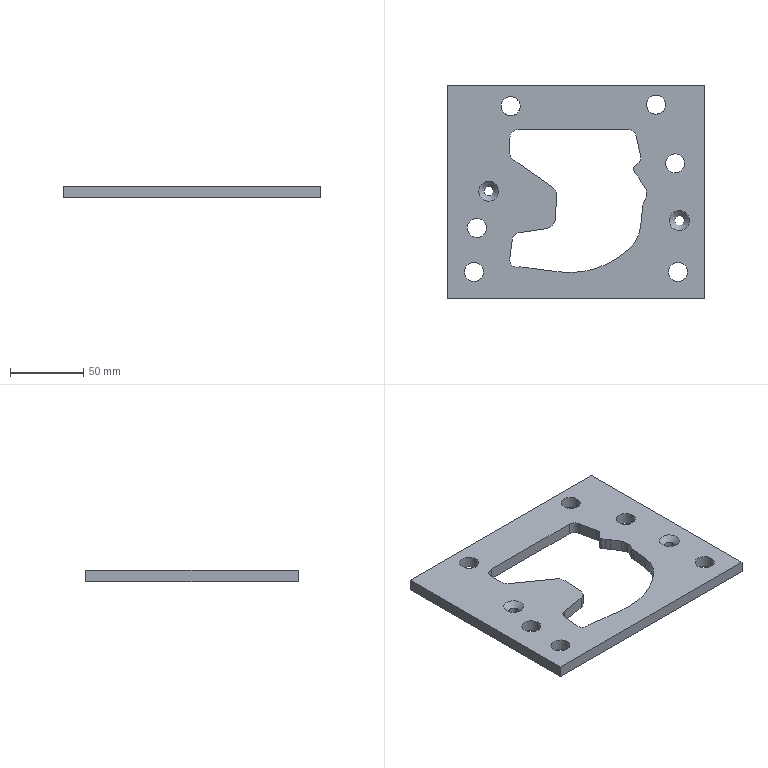Part | STEP file | gslz 2016.10.28-13_id758_x_t | 1 solid | 45 faces | box 175 x 145 x 8 mm | volume 140087 mm3 | plane 22 | cylinder 21 | cone 2 | commonest cylinder face diameters 13 x6 10 x4 14 x3 6.5 x2 4 x1 8 x1